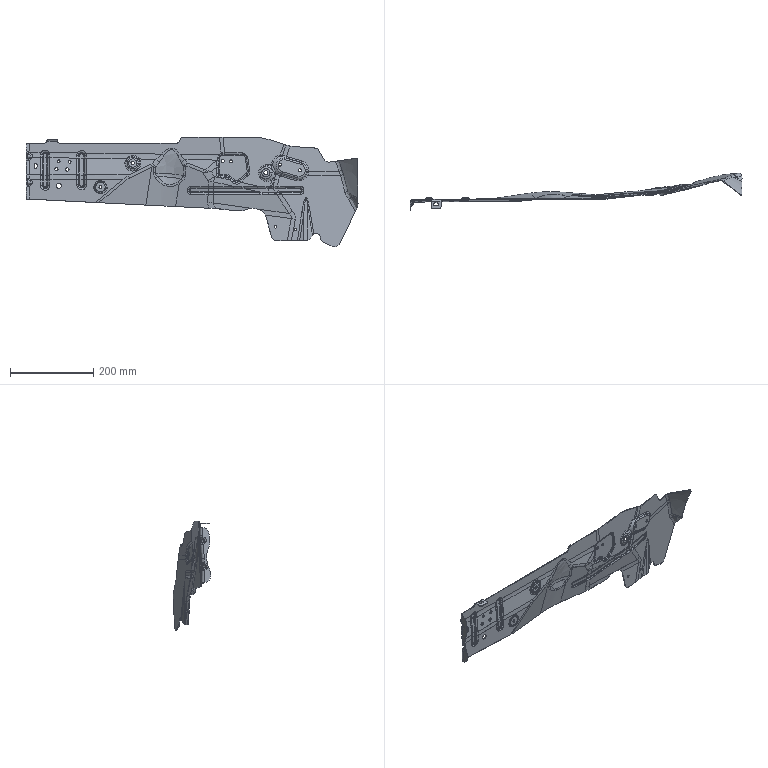Part | 1 solid | 955 faces | box 798.571 x 91.266 x 262.663 mm | volume 209983 mm3 | spline 734 | cylinder 144 | plane 64 | other 7 | sphere 6 | commonest cylinder face diameters 10 x19 13 x12 12 x11 200 x10 7 x9 9 x6